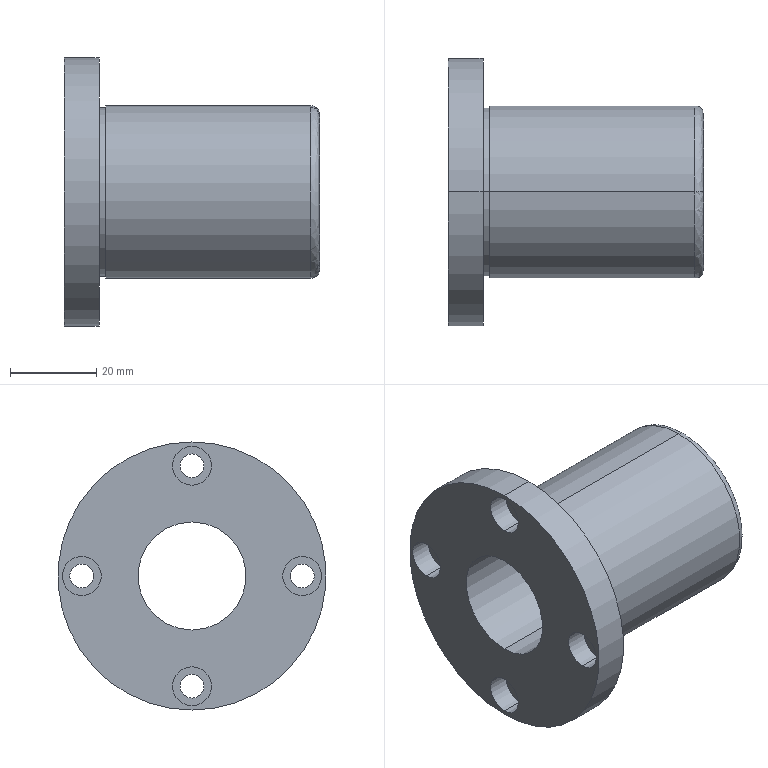Part | SolidWorks | features BaseBody 1 | 1 solid | 34 faces | box 59 x 62 x 62 mm | volume 57509 mm3 | cylinder 24 | plane 8 | spline 2 | commonest cylinder face diameters 5.5 x8 9 x8 25 x2 39 x2 40 x2 62 x2
STEP:
#1=CARTESIAN_POINT('',(57.,0.,-20.));
#2=VERTEX_POINT('',#1);
#3=CARTESIAN_POINT('',(57.,0.,20.));
#4=VERTEX_POINT('',#3);
#5=CARTESIAN_POINT('',(57.,0.,0.));
#6=DIRECTION('',(-1.,0.,0.));
#7=DIRECTION('',(0.,0.,-1.));
#8=AXIS2_PLACEMENT_3D('',#5,#6,#7);
#9=CIRCLE('',#8,20.);
#10=EDGE_CURVE('',#2,#4,#9,.T.);
#11=ORIENTED_EDGE('',*,*,#10,.F.);
#12=CARTESIAN_POINT('',(59.,0.,-18.));
#13=VERTEX_POINT('',#12);
#14=CARTESIAN_POINT('',(57.,0.,-18.));
#15=DIRECTION('',(0.,-1.,0.));
#16=DIRECTION('',(0.,0.,-1.));
#17=AXIS2_PLACEMENT_3D('',#14,#15,#16);
#18=CIRCLE('',#17,2.);
#19=EDGE_CURVE('',#2,#13,#18,.T.);
#20=ORIENTED_EDGE('',*,*,#19,.T.);
#21=CARTESIAN_POINT('',(59.,0.,18.));
#22=VERTEX_POINT('',#21);
#23=CARTESIAN_POINT('',(59.,0.,-18.));
#24=CARTESIAN_POINT('',(59.,-36.,-18.));
#25=CARTESIAN_POINT('',(59.,-36.,18.));
#26=CARTESIAN_POINT('',(59.,0.,18.));
#27=(BOUNDED_CURVE()B_SPLINE_CURVE(3,(#23,#24,#25,#26),.UNSPECIFIED.,.F.,.F.)B_SPLINE_CURVE_WITH_KNOTS((4,4),(0.,1.),.UNSPECIFIED.)CURVE()GEOMETRIC_REPRESENTATION_ITEM()RATIONAL_B_SPLINE_CURVE((1.,0.3333,0.3333,1.))REPRESENTATION_ITEM(''));
#28=EDGE_CURVE('',#13,#22,#27,.T.);
#29=ORIENTED_EDGE('',*,*,#28,.T.);
#30=CARTESIAN_POINT('',(57.,0.,18.));
#31=DIRECTION('',(0.,1.,0.));
#32=DIRECTION('',(0.,0.,1.));
#33=AXIS2_PLACEMENT_3D('',#30,#31,#32);
#34=CIRCLE('',#33,2.);
#35=EDGE_CURVE('',#4,#22,#34,.T.);
#36=ORIENTED_EDGE('',*,*,#35,.F.);
#37=EDGE_LOOP('',(#11,#20,#29,#36));
#38=FACE_OUTER_BOUND('',#37,.T.);
#39=CARTESIAN_POINT('',(57.,0.,-20.));
#40=CARTESIAN_POINT('',(57.,-40.,-20.));
#41=CARTESIAN_POINT('',(57.,-40.,20.));
#42=CARTESIAN_POINT('',(57.,0.,20.));
#43=CARTESIAN_POINT('',(58.172,0.,-20.));
#44=CARTESIAN_POINT('',(58.172,-40.,-20.));
#45=CARTESIAN_POINT('',(58.172,-40.,20.));
#46=CARTESIAN_POINT('',(58.172,0.,20.));
#47=CARTESIAN_POINT('',(59.,0.,-19.172));
#48=CARTESIAN_POINT('',(59.,-38.343,-19.172));
#49=CARTESIAN_POINT('',(59.,-38.343,19.172));
#50=CARTESIAN_POINT('',(59.,0.,19.172));
#51=CARTESIAN_POINT('',(59.,0.,-18.));
#52=CARTESIAN_POINT('',(59.,-36.,-18.));
#53=CARTESIAN_POINT('',(59.,-36.,18.));
#54=CARTESIAN_POINT('',(59.,0.,18.));
#55=(BOUNDED_SURFACE()B_SPLINE_SURFACE(3,3,((#39,#40,#41,#42),(#43,#44,#45,#46),(#47,#48,#49,#50),(#51,#52,#53,#54)),.UNSPECIFIED.,.F.,.F.,.T.)B_SPLINE_SURFACE_WITH_KNOTS((4,4),(4,4),(0.,1.),(0.,1.),.UNSPECIFIED.)GEOMETRIC_REPRESENTATION_ITEM()RATIONAL_B_SPLINE_SURFACE(((1.,0.3333,0.3333,1.),(0.8047,0.2682,0.2682,0.8047),(0.8047,0.2682,0.2682,0.8047),(1.,0.3333,0.3333,1.)))REPRESENTATION_ITEM('')SURFACE());
#56=ADVANCED_FACE('',(#38),#55,.T.);
#57=CARTESIAN_POINT('',(9.5,0.,-20.));
#58=VERTEX_POINT('',#57);
#59=CARTESIAN_POINT('',(9.5,0.,20.));
#60=VERTEX_POINT('',#59);
#61=CARTESIAN_POINT('',(9.5,0.,0.));
#62=DIRECTION('',(1.,0.,0.));
#63=DIRECTION('',(0.,0.,-1.));
#64=AXIS2_PLACEMENT_3D('',#61,#62,#63);
#65=CIRCLE('',#64,20.);
#66=EDGE_CURVE('',#58,#60,#65,.T.);
#67=ORIENTED_EDGE('',*,*,#66,.T.);
#68=CARTESIAN_POINT('',(33.25,0.,20.));
#69=DIRECTION('',(1.,0.,0.));
#70=VECTOR('',#69,1000.);
#71=LINE('',#68,#70);
#72=EDGE_CURVE('',#60,#4,#71,.T.);
#73=ORIENTED_EDGE('',*,*,#72,.T.);
#74=CARTESIAN_POINT('',(57.,0.,0.));
#75=DIRECTION('',(-1.,0.,0.));
#76=DIRECTION('',(0.,0.,-1.));
#77=AXIS2_PLACEMENT_3D('',#74,#75,#76);
#78=CIRCLE('',#77,20.);
#79=EDGE_CURVE('',#4,#2,#78,.T.);
#80=ORIENTED_EDGE('',*,*,#79,.T.);
#81=CARTESIAN_POINT('',(33.25,0.,-20.));
#82=DIRECTION('',(1.,0.,0.));
#83=VECTOR('',#82,1000.);
#84=LINE('',#81,#83);
#85=EDGE_CURVE('',#58,#2,#84,.T.);
#86=ORIENTED_EDGE('',*,*,#85,.F.);
#87=EDGE_LOOP('',(#67,#73,#80,#86));
#88=FACE_OUTER_BOUND('',#87,.T.);
#89=CARTESIAN_POINT('',(33.25,0.,0.));
#90=DIRECTION('',(1.,0.,0.));
#91=DIRECTION('',(0.,0.,-1.));
#92=AXIS2_PLACEMENT_3D('',#89,#90,#91);
#93=CYLINDRICAL_SURFACE('',#92,20.);
#94=ADVANCED_FACE('',(#88),#93,.T.);
#95=CARTESIAN_POINT('',(8.,0.,-19.5));
#96=VERTEX_POINT('',#95);
#97=CARTESIAN_POINT('',(8.,0.,19.5));
#98=VERTEX_POINT('',#97);
#99=CARTESIAN_POINT('',(8.,0.,0.));
#100=DIRECTION('',(1.,0.,0.));
#101=DIRECTION('',(0.,0.,-1.));
#102=AXIS2_PLACEMENT_3D('',#99,#100,#101);
#103=CIRCLE('',#102,19.5);
#104=EDGE_CURVE('',#96,#98,#103,.T.);
#105=ORIENTED_EDGE('',*,*,#104,.T.);
#106=CARTESIAN_POINT('',(9.5,0.,19.5));
#107=VERTEX_POINT('',#106);
#108=CARTESIAN_POINT('',(8.75,0.,19.5));
#109=DIRECTION('',(1.,0.,0.));
#110=VECTOR('',#109,1000.);
#111=LINE('',#108,#110);
#112=EDGE_CURVE('',#98,#107,#111,.T.);
#113=ORIENTED_EDGE('',*,*,#112,.T.);
#114=CARTESIAN_POINT('',(9.5,0.,-19.5));
#115=VERTEX_POINT('',#114);
#116=CARTESIAN_POINT('',(9.5,0.,0.));
#117=DIRECTION('',(1.,0.,0.));
#118=DIRECTION('',(0.,0.,-1.));
#119=AXIS2_PLACEMENT_3D('',#116,#117,#118);
#120=CIRCLE('',#119,19.5);
#121=EDGE_CURVE('',#115,#107,#120,.T.);
#122=ORIENTED_EDGE('',*,*,#121,.F.);
#123=CARTESIAN_POINT('',(8.75,0.,-19.5));
#124=DIRECTION('',(1.,0.,0.));
#125=VECTOR('',#124,1000.);
#126=LINE('',#123,#125);
#127=EDGE_CURVE('',#96,#115,#126,.T.);
#128=ORIENTED_EDGE('',*,*,#127,.F.);
#129=EDGE_LOOP('',(#105,#113,#122,#128));
#130=FACE_OUTER_BOUND('',#129,.T.);
#131=CARTESIAN_POINT('',(8.75,0.,0.));
#132=DIRECTION('',(1.,0.,0.));
#133=DIRECTION('',(0.,0.,-1.));
#134=AXIS2_PLACEMENT_3D('',#131,#132,#133);
#135=CYLINDRICAL_SURFACE('',#134,19.5);
#136=ADVANCED_FACE('',(#130),#135,.T.);
#137=CARTESIAN_POINT('',(0.,0.,12.5));
#138=VERTEX_POINT('',#137);
#139=CARTESIAN_POINT('',(0.,0.,-12.5));
#140=VERTEX_POINT('',#139);
#141=CARTESIAN_POINT('',(0.,0.,0.));
#142=DIRECTION('',(1.,0.,0.));
#143=DIRECTION('',(0.,0.,-1.));
#144=AXIS2_PLACEMENT_3D('',#141,#142,#143);
#145=CIRCLE('',#144,12.5);
#146=EDGE_CURVE('',#138,#140,#145,.T.);
#147=ORIENTED_EDGE('',*,*,#146,.F.);
#148=CARTESIAN_POINT('',(59.,0.,12.5));
#149=VERTEX_POINT('',#148);
#150=CARTESIAN_POINT('',(29.5,0.,12.5));
#151=DIRECTION('',(1.,0.,0.));
#152=VECTOR('',#151,1000.);
#153=LINE('',#150,#152);
#154=EDGE_CURVE('',#138,#149,#153,.T.);
#155=ORIENTED_EDGE('',*,*,#154,.T.);
#156=CARTESIAN_POINT('',(59.,0.,-12.5));
#157=VERTEX_POINT('',#156);
#158=CARTESIAN_POINT('',(59.,0.,0.));
#159=DIRECTION('',(-1.,0.,0.));
#160=DIRECTION('',(0.,0.,-1.));
#161=AXIS2_PLACEMENT_3D('',#158,#159,#160);
#162=CIRCLE('',#161,12.5);
#163=EDGE_CURVE('',#157,#149,#162,.T.);
#164=ORIENTED_EDGE('',*,*,#163,.F.);
#165=CARTESIAN_POINT('',(29.5,0.,-12.5));
#166=DIRECTION('',(1.,0.,0.));
#167=VECTOR('',#166,1000.);
#168=LINE('',#165,#167);
#169=EDGE_CURVE('',#140,#157,#168,.T.);
#170=ORIENTED_EDGE('',*,*,#169,.F.);
#171=EDGE_LOOP('',(#147,#155,#164,#170));
#172=FACE_OUTER_BOUND('',#171,.T.);
#173=CARTESIAN_POINT('',(29.5,0.,0.));
#174=DIRECTION('',(1.,0.,0.));
#175=DIRECTION('',(0.,0.,-1.));
#176=AXIS2_PLACEMENT_3D('',#173,#174,#175);
#177=CYLINDRICAL_SURFACE('',#176,12.5);
#178=ADVANCED_FACE('',(#172),#177,.F.);
#179=CARTESIAN_POINT('',(0.,0.,31.));
#180=VERTEX_POINT('',#179);
#181=CARTESIAN_POINT('',(0.,0.,-31.));
#182=VERTEX_POINT('',#181);
#183=CARTESIAN_POINT('',(0.,0.,0.));
#184=DIRECTION('',(-1.,0.,0.));
#185=DIRECTION('',(0.,0.,-1.));
#186=AXIS2_PLACEMENT_3D('',#183,#184,#185);
#187=CIRCLE('',#186,31.);
#188=EDGE_CURVE('',#180,#182,#187,.T.);
#189=ORIENTED_EDGE('',*,*,#188,.F.);
#190=CARTESIAN_POINT('',(8.,0.,31.));
#191=VERTEX_POINT('',#190);
#192=CARTESIAN_POINT('',(4.,0.,31.));
#193=DIRECTION('',(1.,0.,0.));
#194=VECTOR('',#193,1000.);
#195=LINE('',#192,#194);
#196=EDGE_CURVE('',#180,#191,#195,.T.);
#197=ORIENTED_EDGE('',*,*,#196,.T.);
#198=CARTESIAN_POINT('',(8.,0.,-31.));
#199=VERTEX_POINT('',#198);
#200=CARTESIAN_POINT('',(8.,0.,0.));
#201=DIRECTION('',(1.,0.,0.));
#202=DIRECTION('',(0.,0.,-1.));
#203=AXIS2_PLACEMENT_3D('',#200,#201,#202);
#204=CIRCLE('',#203,31.);
#205=EDGE_CURVE('',#199,#191,#204,.T.);
#206=ORIENTED_EDGE('',*,*,#205,.F.);
#207=CARTESIAN_POINT('',(4.,0.,-31.));
#208=DIRECTION('',(1.,0.,0.));
#209=VECTOR('',#208,1000.);
#210=LINE('',#207,#209);
#211=EDGE_CURVE('',#182,#199,#210,.T.);
#212=ORIENTED_EDGE('',*,*,#211,.F.);
#213=EDGE_LOOP('',(#189,#197,#206,#212));
#214=FACE_OUTER_BOUND('',#213,.T.);
#215=CARTESIAN_POINT('',(4.,0.,0.));
#216=DIRECTION('',(1.,0.,0.));
#217=DIRECTION('',(0.,0.,-1.));
#218=AXIS2_PLACEMENT_3D('',#215,#216,#217);
#219=CYLINDRICAL_SURFACE('',#218,31.);
#220=ADVANCED_FACE('',(#214),#219,.T.);
#221=CARTESIAN_POINT('',(5.1,25.5,2.75));
#222=VERTEX_POINT('',#221);
#223=CARTESIAN_POINT('',(5.1,25.5,-2.75));
#224=VERTEX_POINT('',#223);
#225=CARTESIAN_POINT('',(5.1,25.5,0.));
#226=DIRECTION('',(1.,0.,0.));
#227=DIRECTION('',(0.,0.,-1.));
#228=AXIS2_PLACEMENT_3D('',#225,#226,#227);
#229=CIRCLE('',#228,2.75);
#230=EDGE_CURVE('',#222,#224,#229,.T.);
#231=ORIENTED_EDGE('',*,*,#230,.F.);
#232=CARTESIAN_POINT('',(8.,25.5,2.75));
#233=VERTEX_POINT('',#232);
#234=CARTESIAN_POINT('',(6.55,25.5,2.75));
#235=DIRECTION('',(1.,0.,0.));
#236=VECTOR('',#235,1000.);
#237=LINE('',#234,#236);
#238=EDGE_CURVE('',#222,#233,#237,.T.);
#239=ORIENTED_EDGE('',*,*,#238,.T.);
#240=CARTESIAN_POINT('',(8.,25.5,-2.75));
#241=VERTEX_POINT('',#240);
#242=CARTESIAN_POINT('',(8.,25.5,0.));
#243=DIRECTION('',(-1.,0.,0.));
#244=DIRECTION('',(0.,0.,-1.));
#245=AXIS2_PLACEMENT_3D('',#242,#243,#244);
#246=CIRCLE('',#245,2.75);
#247=EDGE_CURVE('',#241,#233,#246,.T.);
#248=ORIENTED_EDGE('',*,*,#247,.F.);
#249=CARTESIAN_POINT('',(6.55,25.5,-2.75));
#250=DIRECTION('',(1.,0.,0.));
#251=VECTOR('',#250,1000.);
#252=LINE('',#249,#251);
#253=EDGE_CURVE('',#224,#241,#252,.T.);
#254=ORIENTED_EDGE('',*,*,#253,.F.);
#255=EDGE_LOOP('',(#231,#239,#248,#254));
#256=FACE_OUTER_BOUND('',#255,.T.);
#257=CARTESIAN_POINT('',(6.55,25.5,0.));
#258=DIRECTION('',(1.,0.,0.));
#259=DIRECTION('',(0.,0.,-1.));
#260=AXIS2_PLACEMENT_3D('',#257,#258,#259);
#261=CYLINDRICAL_SURFACE('',#260,2.75);
#262=ADVANCED_FACE('',(#256),#261,.F.);
#263=CARTESIAN_POINT('',(5.1,-25.5,2.75));
#264=VERTEX_POINT('',#263);
#265=CARTESIAN_POINT('',(5.1,-25.5,-2.75));
#266=VERTEX_POINT('',#265);
#267=CARTESIAN_POINT('',(5.1,-25.5,0.));
#268=DIRECTION('',(1.,0.,0.));
#269=DIRECTION('',(0.,0.,-1.));
#270=AXIS2_PLACEMENT_3D('',#267,#268,#269);
#271=CIRCLE('',#270,2.75);
#272=EDGE_CURVE('',#264,#266,#271,.T.);
#273=ORIENTED_EDGE('',*,*,#272,.F.);
#274=CARTESIAN_POINT('',(8.,-25.5,2.75));
#275=VERTEX_POINT('',#274);
#276=CARTESIAN_POINT('',(6.55,-25.5,2.75));
#277=DIRECTION('',(1.,0.,0.));
#278=VECTOR('',#277,1000.);
#279=LINE('',#276,#278);
#280=EDGE_CURVE('',#264,#275,#279,.T.);
#281=ORIENTED_EDGE('',*,*,#280,.T.);
#282=CARTESIAN_POINT('',(8.,-25.5,-2.75));
#283=VERTEX_POINT('',#282);
#284=CARTESIAN_POINT('',(8.,-25.5,0.));
#285=DIRECTION('',(-1.,0.,0.));
#286=DIRECTION('',(0.,0.,-1.));
#287=AXIS2_PLACEMENT_3D('',#284,#285,#286);
#288=CIRCLE('',#287,2.75);
#289=EDGE_CURVE('',#283,#275,#288,.T.);
#290=ORIENTED_EDGE('',*,*,#289,.F.);
#291=CARTESIAN_POINT('',(6.55,-25.5,-2.75));
#292=DIRECTION('',(1.,0.,0.));
#293=VECTOR('',#292,1000.);
#294=LINE('',#291,#293);
#295=EDGE_CURVE('',#266,#283,#294,.T.);
#296=ORIENTED_EDGE('',*,*,#295,.F.);
#297=EDGE_LOOP('',(#273,#281,#290,#296));
#298=FACE_OUTER_BOUND('',#297,.T.);
#299=CARTESIAN_POINT('',(6.55,-25.5,0.));
#300=DIRECTION('',(1.,0.,0.));
#301=DIRECTION('',(0.,0.,-1.));
#302=AXIS2_PLACEMENT_3D('',#299,#300,#301);
#303=CYLINDRICAL_SURFACE('',#302,2.75);
#304=ADVANCED_FACE('',(#298),#303,.F.);
#305=CARTESIAN_POINT('',(5.1,0.,-22.75));
#306=VERTEX_POINT('',#305);
#307=CARTESIAN_POINT('',(5.1,0.,-28.25));
#308=VERTEX_POINT('',#307);
#309=CARTESIAN_POINT('',(5.1,0.,-25.5));
#310=DIRECTION('',(1.,0.,0.));
#311=DIRECTION('',(0.,0.,-1.));
#312=AXIS2_PLACEMENT_3D('',#309,#310,#311);
#313=CIRCLE('',#312,2.75);
#314=EDGE_CURVE('',#306,#308,#313,.T.);
#315=ORIENTED_EDGE('',*,*,#314,.F.);
#316=CARTESIAN_POINT('',(8.,0.,-22.75));
#317=VERTEX_POINT('',#316);
#318=CARTESIAN_POINT('',(6.55,0.,-22.75));
#319=DIRECTION('',(1.,0.,0.));
#320=VECTOR('',#319,1000.);
#321=LINE('',#318,#320);
#322=EDGE_CURVE('',#306,#317,#321,.T.);
#323=ORIENTED_EDGE('',*,*,#322,.T.);
#324=CARTESIAN_POINT('',(8.,0.,-28.25));
#325=VERTEX_POINT('',#324);
#326=CARTESIAN_POINT('',(8.,0.,-25.5));
#327=DIRECTION('',(-1.,0.,0.));
#328=DIRECTION('',(0.,0.,-1.));
#329=AXIS2_PLACEMENT_3D('',#326,#327,#328);
#330=CIRCLE('',#329,2.75);
#331=EDGE_CURVE('',#325,#317,#330,.T.);
#332=ORIENTED_EDGE('',*,*,#331,.F.);
#333=CARTESIAN_POINT('',(6.55,0.,-28.25));
#334=DIRECTION('',(1.,0.,0.));
#335=VECTOR('',#334,1000.);
#336=LINE('',#333,#335);
#337=EDGE_CURVE('',#308,#325,#336,.T.);
#338=ORIENTED_EDGE('',*,*,#337,.F.);
#339=EDGE_LOOP('',(#315,#323,#332,#338));
#340=FACE_OUTER_BOUND('',#339,.T.);
#341=CARTESIAN_POINT('',(6.55,0.,-25.5));
#342=DIRECTION('',(1.,0.,0.));
#343=DIRECTION('',(0.,0.,-1.));
#344=AXIS2_PLACEMENT_3D('',#341,#342,#343);
#345=CYLINDRICAL_SURFACE('',#344,2.75);
#346=ADVANCED_FACE('',(#340),#345,.F.);
#347=CARTESIAN_POINT('',(5.1,0.,28.25));
#348=VERTEX_POINT('',#347);
#349=CARTESIAN_POINT('',(5.1,0.,22.75));
#350=VERTEX_POINT('',#349);
#351=CARTESIAN_POINT('',(5.1,0.,25.5));
#352=DIRECTION('',(1.,0.,0.));
#353=DIRECTION('',(0.,0.,-1.));
#354=AXIS2_PLACEMENT_3D('',#351,#352,#353);
#355=CIRCLE('',#354,2.75);
#356=EDGE_CURVE('',#348,#350,#355,.T.);
#357=ORIENTED_EDGE('',*,*,#356,.F.);
#358=CARTESIAN_POINT('',(8.,0.,28.25));
#359=VERTEX_POINT('',#358);
#360=CARTESIAN_POINT('',(6.55,0.,28.25));
#361=DIRECTION('',(1.,0.,0.));
#362=VECTOR('',#361,1000.);
#363=LINE('',#360,#362);
#364=EDGE_CURVE('',#348,#359,#363,.T.);
#365=ORIENTED_EDGE('',*,*,#364,.T.);
#366=CARTESIAN_POINT('',(8.,0.,22.75));
#367=VERTEX_POINT('',#366);
#368=CARTESIAN_POINT('',(8.,0.,25.5));
#369=DIRECTION('',(-1.,0.,0.));
#370=DIRECTION('',(0.,0.,-1.));
#371=AXIS2_PLACEMENT_3D('',#368,#369,#370);
#372=CIRCLE('',#371,2.75);
#373=EDGE_CURVE('',#367,#359,#372,.T.);
#374=ORIENTED_EDGE('',*,*,#373,.F.);
#375=CARTESIAN_POINT('',(6.55,0.,22.75));
#376=DIRECTION('',(1.,0.,0.));
#377=VECTOR('',#376,1000.);
#378=LINE('',#375,#377);
#379=EDGE_CURVE('',#350,#367,#378,.T.);
#380=ORIENTED_EDGE('',*,*,#379,.F.);
#381=EDGE_LOOP('',(#357,#365,#374,#380));
#382=FACE_OUTER_BOUND('',#381,.T.);
#383=CARTESIAN_POINT('',(6.55,0.,25.5));
#384=DIRECTION('',(1.,0.,0.));
#385=DIRECTION('',(0.,0.,-1.));
#386=AXIS2_PLACEMENT_3D('',#383,#384,#385);
#387=CYLINDRICAL_SURFACE('',#386,2.75);
#388=ADVANCED_FACE('',(#382),#387,.F.);
#389=CARTESIAN_POINT('',(0.,25.5,4.5));
#390=VERTEX_POINT('',#389);
#391=CARTESIAN_POINT('',(0.,25.5,-4.5));
#392=VERTEX_POINT('',#391);
#393=CARTESIAN_POINT('',(0.,25.5,0.));
#394=DIRECTION('',(1.,0.,0.));
#395=DIRECTION('',(0.,0.,-1.));
#396=AXIS2_PLACEMENT_3D('',#393,#394,#395);
#397=CIRCLE('',#396,4.5);
#398=EDGE_CURVE('',#390,#392,#397,.T.);
#399=ORIENTED_EDGE('',*,*,#398,.F.);
#400=CARTESIAN_POINT('',(5.1,25.5,4.5));
#401=VERTEX_POINT('',#400);
#402=CARTESIAN_POINT('',(2.55,25.5,4.5));
#403=DIRECTION('',(1.,0.,0.));
#404=VECTOR('',#403,1000.);
#405=LINE('',#402,#404);
#406=EDGE_CURVE('',#390,#401,#405,.T.);
#407=ORIENTED_EDGE('',*,*,#406,.T.);
#408=CARTESIAN_POINT('',(5.1,25.5,-4.5));
#409=VERTEX_POINT('',#408);
#410=CARTESIAN_POINT('',(5.1,25.5,0.));
#411=DIRECTION('',(-1.,0.,0.));
#412=DIRECTION('',(0.,0.,-1.));
#413=AXIS2_PLACEMENT_3D('',#410,#411,#412);
#414=CIRCLE('',#413,4.5);
#415=EDGE_CURVE('',#409,#401,#414,.T.);
#416=ORIENTED_EDGE('',*,*,#415,.F.);
#417=CARTESIAN_POINT('',(2.55,25.5,-4.5));
#418=DIRECTION('',(1.,0.,0.));
#419=VECTOR('',#418,1000.);
#420=LINE('',#417,#419);
#421=EDGE_CURVE('',#392,#409,#420,.T.);
#422=ORIENTED_EDGE('',*,*,#421,.F.);
#423=EDGE_LOOP('',(#399,#407,#416,#422));
#424=FACE_OUTER_BOUND('',#423,.T.);
#425=CARTESIAN_POINT('',(2.55,25.5,0.));
#426=DIRECTION('',(1.,0.,0.));
#427=DIRECTION('',(0.,0.,-1.));
#428=AXIS2_PLACEMENT_3D('',#425,#426,#427);
#429=CYLINDRICAL_SURFACE('',#428,4.5);
#430=ADVANCED_FACE('',(#424),#429,.F.);
#431=CARTESIAN_POINT('',(0.,-25.5,4.5));
#432=VERTEX_POINT('',#431);
#433=CARTESIAN_POINT('',(0.,-25.5,-4.5));
#434=VERTEX_POINT('',#433);
#435=CARTESIAN_POINT('',(0.,-25.5,0.));
#436=DIRECTION('',(1.,0.,0.));
#437=DIRECTION('',(0.,0.,-1.));
#438=AXIS2_PLACEMENT_3D('',#435,#436,#437);
#439=CIRCLE('',#438,4.5);
#440=EDGE_CURVE('',#432,#434,#439,.T.);
#441=ORIENTED_EDGE('',*,*,#440,.F.);
#442=CARTESIAN_POINT('',(5.1,-25.5,4.5));
#443=VERTEX_POINT('',#442);
#444=CARTESIAN_POINT('',(2.55,-25.5,4.5));
#445=DIRECTION('',(1.,0.,0.));
#446=VECTOR('',#445,1000.);
#447=LINE('',#444,#446);
#448=EDGE_CURVE('',#432,#443,#447,.T.);
#449=ORIENTED_EDGE('',*,*,#448,.T.);
#450=CARTESIAN_POINT('',(5.1,-25.5,-4.5));
#451=VERTEX_POINT('',#450);
#452=CARTESIAN_POINT('',(5.1,-25.5,0.));
#453=DIRECTION('',(-1.,0.,0.));
#454=DIRECTION('',(0.,0.,-1.));
#455=AXIS2_PLACEMENT_3D('',#452,#453,#454);
#456=CIRCLE('',#455,4.5);
#457=EDGE_CURVE('',#451,#443,#456,.T.);
#458=ORIENTED_EDGE('',*,*,#457,.F.);
#459=CARTESIAN_POINT('',(2.55,-25.5,-4.5));
#460=DIRECTION('',(1.,0.,0.));
#461=VECTOR('',#460,1000.);
#462=LINE('',#459,#461);
#463=EDGE_CURVE('',#434,#451,#462,.T.);
#464=ORIENTED_EDGE('',*,*,#463,.F.);
#465=EDGE_LOOP('',(#441,#449,#458,#464));
#466=FACE_OUTER_BOUND('',#465,.T.);
#467=CARTESIAN_POINT('',(2.55,-25.5,0.));
#468=DIRECTION('',(1.,0.,0.));
#469=DIRECTION('',(0.,0.,-1.));
#470=AXIS2_PLACEMENT_3D('',#467,#468,#469);
#471=CYLINDRICAL_SURFACE('',#470,4.5);
#472=ADVANCED_FACE('',(#466),#471,.F.);
#473=CARTESIAN_POINT('',(0.,0.,-21.));
#474=VERTEX_POINT('',#473);
#475=CARTESIAN_POINT('',(0.,0.,-30.));
#476=VERTEX_POINT('',#475);
#477=CARTESIAN_POINT('',(0.,0.,-25.5));
#478=DIRECTION('',(1.,0.,0.));
#479=DIRECTION('',(0.,0.,-1.));
#480=AXIS2_PLACEMENT_3D('',#477,#478,#479);
#481=CIRCLE('',#480,4.5);
#482=EDGE_CURVE('',#474,#476,#481,.T.);
#483=ORIENTED_EDGE('',*,*,#482,.F.);
#484=CARTESIAN_POINT('',(5.1,0.,-21.));
#485=VERTEX_POINT('',#484);
#486=CARTESIAN_POINT('',(2.55,0.,-21.));
#487=DIRECTION('',(1.,0.,0.));
#488=VECTOR('',#487,1000.);
#489=LINE('',#486,#488);
#490=EDGE_CURVE('',#474,#485,#489,.T.);
#491=ORIENTED_EDGE('',*,*,#490,.T.);
#492=CARTESIAN_POINT('',(5.1,0.,-30.));
#493=VERTEX_POINT('',#492);
#494=CARTESIAN_POINT('',(5.1,0.,-25.5));
#495=DIRECTION('',(-1.,0.,0.));
#496=DIRECTION('',(0.,0.,-1.));
#497=AXIS2_PLACEMENT_3D('',#494,#495,#496);
#498=CIRCLE('',#497,4.5);
#499=EDGE_CURVE('',#493,#485,#498,.T.);
#500=ORIENTED_EDGE('',*,*,#499,.F.);
#501=CARTESIAN_POINT('',(2.55,0.,-30.));
#502=DIRECTION('',(1.,0.,0.));
#503=VECTOR('',#502,1000.);
#504=LINE('',#501,#503);
#505=EDGE_CURVE('',#476,#493,#504,.T.);
#506=ORIENTED_EDGE('',*,*,#505,.F.);
#507=EDGE_LOOP('',(#483,#491,#500,#506));
#508=FACE_OUTER_BOUND('',#507,.T.);
#509=CARTESIAN_POINT('',(2.55,0.,-25.5));
#510=DIRECTION('',(1.,0.,0.));
#511=DIRECTION('',(0.,0.,-1.));
#512=AXIS2_PLACEMENT_3D('',#509,#510,#511);
#513=CYLINDRICAL_SURFACE('',#512,4.5);
#514=ADVANCED_FACE('',(#508),#513,.F.);
#515=CARTESIAN_POINT('',(0.,0.,30.));
#516=VERTEX_POINT('',#515);
#517=CARTESIAN_POINT('',(0.,0.,21.));
#518=VERTEX_POINT('',#517);
#519=CARTESIAN_POINT('',(0.,0.,25.5));
#520=DIRECTION('',(1.,0.,0.));
#521=DIRECTION('',(0.,0.,-1.));
#522=AXIS2_PLACEMENT_3D('',#519,#520,#521);
#523=CIRCLE('',#522,4.5);
#524=EDGE_CURVE('',#516,#518,#523,.T.);
#525=ORIENTED_EDGE('',*,*,#524,.F.);
#526=CARTESIAN_POINT('',(5.1,0.,30.));
#527=VERTEX_POINT('',#526);
#528=CARTESIAN_POINT('',(2.55,0.,30.));
#529=DIRECTION('',(1.,0.,0.));
#530=VECTOR('',#529,1000.);
#531=LINE('',#528,#530);
#532=EDGE_CURVE('',#516,#527,#531,.T.);
#533=ORIENTED_EDGE('',*,*,#532,.T.);
#534=CARTESIAN_POINT('',(5.1,0.,21.));
#535=VERTEX_POINT('',#534);
#536=CARTESIAN_POINT('',(5.1,0.,25.5));
#537=DIRECTION('',(-1.,0.,0.));
#538=DIRECTION('',(0.,0.,-1.));
#539=AXIS2_PLACEMENT_3D('',#536,#537,#538);
#540=CIRCLE('',#539,4.5);
#541=EDGE_CURVE('',#535,#527,#540,.T.);
#542=ORIENTED_EDGE('',*,*,#541,.F.);
#543=CARTESIAN_POINT('',(2.55,0.,21.));
#544=DIRECTION('',(1.,0.,0.));
#545=VECTOR('',#544,1000.);
#546=LINE('',#543,#545);
#547=EDGE_CURVE('',#518,#535,#546,.T.);
#548=ORIENTED_EDGE('',*,*,#547,.F.);
#549=EDGE_LOOP('',(#525,#533,#542,#548));
#550=FACE_OUTER_BOUND('',#549,.T.);
#551=CARTESIAN_POINT('',(2.55,0.,25.5));
#552=DIRECTION('',(1.,0.,0.));
#553=DIRECTION('',(0.,0.,-1.));
#554=AXIS2_PLACEMENT_3D('',#551,#552,#553);
#555=CYLINDRICAL_SURFACE('',#554,4.5);
#556=ADVANCED_FACE('',(#550),#555,.F.);
#557=ORIENTED_EDGE('',*,*,#72,.F.);
#558=CARTESIAN_POINT('',(9.5,0.,0.));
#559=DIRECTION('',(1.,0.,0.));
#560=DIRECTION('',(0.,0.,-1.));
#561=AXIS2_PLACEMENT_3D('',#558,#559,#560);
#562=CIRCLE('',#561,20.);
#563=EDGE_CURVE('',#60,#58,#562,.T.);
#564=ORIENTED_EDGE('',*,*,#563,.T.);
#565=ORIENTED_EDGE('',*,*,#85,.T.);
#566=ORIENTED_EDGE('',*,*,#10,.T.);
#567=EDGE_LOOP('',(#557,#564,#565,#566));
#568=FACE_OUTER_BOUND('',#567,.T.);
#569=CARTESIAN_POINT('',(33.25,0.,0.));
#570=DIRECTION('',(1.,0.,0.));
#571=DIRECTION('',(0.,0.,-1.));
#572=AXIS2_PLACEMENT_3D('',#569,#570,#571);
#573=CYLINDRICAL_SURFACE('',#572,20.);
#574=ADVANCED_FACE('',(#568),#573,.T.);
#575=ORIENTED_EDGE('',*,*,#19,.F.);
#576=ORIENTED_EDGE('',*,*,#79,.F.);
#577=ORIENTED_EDGE('',*,*,#35,.T.);
#578=CARTESIAN_POINT('',(59.,18.,0.));
#579=VERTEX_POINT('',#578);
#580=CARTESIAN_POINT('',(59.,0.,18.));
#581=CARTESIAN_POINT('',(59.,10.544,18.));
#582=CARTESIAN_POINT('',(59.,18.,10.544));
#583=CARTESIAN_POINT('',(59.,18.,0.));
#584=(BOUNDED_CURVE()B_SPLINE_CURVE(3,(#580,#581,#582,#583),.UNSPECIFIED.,.F.,.F.)B_SPLINE_CURVE_WITH_KNOTS((4,4),(0.,1.),.UNSPECIFIED.)CURVE()GEOMETRIC_REPRESENTATION_ITEM()RATIONAL_B_SPLINE_CURVE((1.,0.8047,0.8047,1.))REPRESENTATION_ITEM(''));
#585=EDGE_CURVE('',#22,#579,#584,.T.);
#586=ORIENTED_EDGE('',*,*,#585,.T.);
#587=CARTESIAN_POINT('',(59.,18.,0.));
#588=CARTESIAN_POINT('',(59.,18.,-10.544));
#589=CARTESIAN_POINT('',(59.,10.544,-18.));
#590=CARTESIAN_POINT('',(59.,0.,-18.));
#591=(BOUNDED_CURVE()B_SPLINE_CURVE(3,(#587,#588,#589,#590),.UNSPECIFIED.,.F.,.F.)B_SPLINE_CURVE_WITH_KNOTS((4,4),(0.,1.),.UNSPECIFIED.)CURVE()GEOMETRIC_REPRESENTATION_ITEM()RATIONAL_B_SPLINE_CURVE((1.,0.8047,0.8047,1.))REPRESENTATION_ITEM(''));
#592=EDGE_CURVE('',#579,#13,#591,.T.);
#593=ORIENTED_EDGE('',*,*,#592,.T.);
#594=EDGE_LOOP('',(#575,#576,#577,#586,#593));
#595=FACE_OUTER_BOUND('',#594,.T.);
#596=CARTESIAN_POINT('',(57.,0.,20.));
#597=CARTESIAN_POINT('',(57.,40.,20.));
#598=CARTESIAN_POINT('',(57.,40.,-20.));
#599=CARTESIAN_POINT('',(57.,0.,-20.));
#600=CARTESIAN_POINT('',(58.172,0.,20.));
#601=CARTESIAN_POINT('',(58.172,40.,20.));
#602=CARTESIAN_POINT('',(58.172,40.,-20.));
#603=CARTESIAN_POINT('',(58.172,0.,-20.));
#604=CARTESIAN_POINT('',(59.,0.,19.172));
#605=CARTESIAN_POINT('',(59.,38.343,19.172));
#606=CARTESIAN_POINT('',(59.,38.343,-19.172));
#607=CARTESIAN_POINT('',(59.,0.,-19.172));
#608=CARTESIAN_POINT('',(59.,0.,18.));
#609=CARTESIAN_POINT('',(59.,36.,18.));
#610=CARTESIAN_POINT('',(59.,36.,-18.));
#611=CARTESIAN_POINT('',(59.,0.,-18.));
#612=(BOUNDED_SURFACE()B_SPLINE_SURFACE(3,3,((#596,#597,#598,#599),(#600,#601,#602,#603),(#604,#605,#606,#607),(#608,#609,#610,#611)),.UNSPECIFIED.,.F.,.F.,.T.)B_SPLINE_SURFACE_WITH_KNOTS((4,4),(4,4),(0.,1.),(0.,1.),.UNSPECIFIED.)GEOMETRIC_REPRESENTATION_ITEM()RATIONAL_B_SPLINE_SURFACE(((1.,0.3333,0.3333,1.),(0.8047,0.2682,0.2682,0.8047),(0.8047,0.2682,0.2682,0.8047),(1.,0.3333,0.3333,1.)))REPRESENTATION_ITEM('')SURFACE());
#613=ADVANCED_FACE('',(#595),#612,.T.);
#614=ORIENTED_EDGE('',*,*,#66,.F.);
#615=ORIENTED_EDGE('',*,*,#563,.F.);
#616=EDGE_LOOP('',(#614,#615));
#617=FACE_OUTER_BOUND('',#616,.T.);
#618=ORIENTED_EDGE('',*,*,#121,.T.);
#619=CARTESIAN_POINT('',(9.5,0.,0.));
#620=DIRECTION('',(1.,0.,0.));
#621=DIRECTION('',(0.,0.,-1.));
#622=AXIS2_PLACEMENT_3D('',#619,#620,#621);
#623=CIRCLE('',#622,19.5);
#624=EDGE_CURVE('',#107,#115,#623,.T.);
#625=ORIENTED_EDGE('',*,*,#624,.T.);
#626=EDGE_LOOP('',(#618,#625));
#627=FACE_BOUND('',#626,.T.);
#628=CARTESIAN_POINT('',(9.5,19.75,0.));
#629=DIRECTION('',(-1.,0.,0.));
#630=DIRECTION('',(0.,0.,1.));
#631=AXIS2_PLACEMENT_3D('',#628,#629,#630);
#632=PLANE('',#631);
#633=ADVANCED_FACE('',(#617,#627),#632,.T.);
#634=ORIENTED_EDGE('',*,*,#163,.T.);
#635=CARTESIAN_POINT('',(59.,0.,0.));
#636=DIRECTION('',(-1.,0.,0.));
#637=DIRECTION('',(0.,0.,-1.));
#638=AXIS2_PLACEMENT_3D('',#635,#636,#637);
#639=CIRCLE('',#638,12.5);
#640=EDGE_CURVE('',#149,#157,#639,.T.);
#641=ORIENTED_EDGE('',*,*,#640,.T.);
#642=EDGE_LOOP('',(#634,#641));
#643=FACE_BOUND('',#642,.T.);
#644=ORIENTED_EDGE('',*,*,#585,.F.);
#645=ORIENTED_EDGE('',*,*,#28,.F.);
#646=ORIENTED_EDGE('',*,*,#592,.F.);
#647=EDGE_LOOP('',(#644,#645,#646));
#648=FACE_OUTER_BOUND('',#647,.T.);
#649=CARTESIAN_POINT('',(59.,15.25,0.));
#650=DIRECTION('',(1.,0.,0.));
#651=DIRECTION('',(0.,0.,-1.));
#652=AXIS2_PLACEMENT_3D('',#649,#650,#651);
#653=PLANE('',#652);
#654=ADVANCED_FACE('',(#643,#648),#653,.T.);
#655=ORIENTED_EDGE('',*,*,#112,.F.);
#656=CARTESIAN_POINT('',(8.,0.,0.));
#657=DIRECTION('',(1.,0.,0.));
#658=DIRECTION('',(0.,0.,-1.));
#659=AXIS2_PLACEMENT_3D('',#656,#657,#658);
#660=CIRCLE('',#659,19.5);
#661=EDGE_CURVE('',#98,#96,#660,.T.);
#662=ORIENTED_EDGE('',*,*,#661,.T.);
#663=ORIENTED_EDGE('',*,*,#127,.T.);
#664=ORIENTED_EDGE('',*,*,#624,.F.);
#665=EDGE_LOOP('',(#655,#662,#663,#664));
#666=FACE_OUTER_BOUND('',#665,.T.);
#667=CARTESIAN_POINT('',(8.75,0.,0.));
#668=DIRECTION('',(1.,0.,0.));
#669=DIRECTION('',(0.,0.,-1.));
#670=AXIS2_PLACEMENT_3D('',#667,#668,#669);
#671=CYLINDRICAL_SURFACE('',#670,19.5);
#672=ADVANCED_FACE('',(#666),#671,.T.);
#673=ORIENTED_EDGE('',*,*,#154,.F.);
#674=CARTESIAN_POINT('',(0.,0.,0.));
#675=DIRECTION('',(1.,0.,0.));
#676=DIRECTION('',(0.,0.,-1.));
#677=AXIS2_PLACEMENT_3D('',#674,#675,#676);
#678=CIRCLE('',#677,12.5);
#679=EDGE_CURVE('',#140,#138,#678,.T.);
#680=ORIENTED_EDGE('',*,*,#679,.F.);
#681=ORIENTED_EDGE('',*,*,#169,.T.);
#682=ORIENTED_EDGE('',*,*,#640,.F.);
#683=EDGE_LOOP('',(#673,#680,#681,#682));
#684=FACE_OUTER_BOUND('',#683,.T.);
#685=CARTESIAN_POINT('',(29.5,0.,0.));
#686=DIRECTION('',(1.,0.,0.));
#687=DIRECTION('',(0.,0.,-1.));
#688=AXIS2_PLACEMENT_3D('',#685,#686,#687);
#689=CYLINDRICAL_SURFACE('',#688,12.5);
#690=ADVANCED_FACE('',(#684),#689,.F.);
#691=ORIENTED_EDGE('',*,*,#104,.F.);
#692=ORIENTED_EDGE('',*,*,#661,.F.);
#693=EDGE_LOOP('',(#691,#692));
#694=FACE_BOUND('',#693,.T.);
#695=ORIENTED_EDGE('',*,*,#205,.T.);
#696=CARTESIAN_POINT('',(8.,0.,0.));
#697=DIRECTION('',(1.,0.,0.));
#698=DIRECTION('',(0.,0.,-1.));
#699=AXIS2_PLACEMENT_3D('',#696,#697,#698);
#700=CIRCLE('',#699,31.);
#701=EDGE_CURVE('',#191,#199,#700,.T.);
#702=ORIENTED_EDGE('',*,*,#701,.T.);
#703=EDGE_LOOP('',(#695,#702));
#704=FACE_OUTER_BOUND('',#703,.T.);
#705=ORIENTED_EDGE('',*,*,#247,.T.);
#706=CARTESIAN_POINT('',(8.,25.5,0.));
#707=DIRECTION('',(-1.,0.,0.));
#708=DIRECTION('',(0.,0.,-1.));
#709=AXIS2_PLACEMENT_3D('',#706,#707,#708);
#710=CIRCLE('',#709,2.75);
#711=EDGE_CURVE('',#233,#241,#710,.T.);
#712=ORIENTED_EDGE('',*,*,#711,.T.);
#713=EDGE_LOOP('',(#705,#712));
#714=FACE_BOUND('',#713,.T.);
#715=ORIENTED_EDGE('',*,*,#289,.T.);
#716=CARTESIAN_POINT('',(8.,-25.5,0.));
#717=DIRECTION('',(-1.,0.,0.));
#718=DIRECTION('',(0.,0.,-1.));
#719=AXIS2_PLACEMENT_3D('',#716,#717,#718);
#720=CIRCLE('',#719,2.75);
#721=EDGE_CURVE('',#275,#283,#720,.T.);
#722=ORIENTED_EDGE('',*,*,#721,.T.);
#723=EDGE_LOOP('',(#715,#722));
#724=FACE_BOUND('',#723,.T.);
#725=ORIENTED_EDGE('',*,*,#331,.T.);
#726=CARTESIAN_POINT('',(8.,0.,-25.5));
#727=DIRECTION('',(-1.,0.,0.));
#728=DIRECTION('',(0.,0.,-1.));
#729=AXIS2_PLACEMENT_3D('',#726,#727,#728);
#730=CIRCLE('',#729,2.75);
#731=EDGE_CURVE('',#317,#325,#730,.T.);
#732=ORIENTED_EDGE('',*,*,#731,.T.);
#733=EDGE_LOOP('',(#725,#732));
#734=FACE_BOUND('',#733,.T.);
#735=ORIENTED_EDGE('',*,*,#373,.T.);
#736=CARTESIAN_POINT('',(8.,0.,25.5));
#737=DIRECTION('',(-1.,0.,0.));
#738=DIRECTION('',(0.,0.,-1.));
#739=AXIS2_PLACEMENT_3D('',#736,#737,#738);
#740=CIRCLE('',#739,2.75);
#741=EDGE_CURVE('',#359,#367,#740,.T.);
#742=ORIENTED_EDGE('',*,*,#741,.T.);
#743=EDGE_LOOP('',(#735,#742));
#744=FACE_BOUND('',#743,.T.);
#745=CARTESIAN_POINT('',(8.,25.25,0.));
#746=DIRECTION('',(1.,0.,0.));
#747=DIRECTION('',(0.,0.,-1.));
#748=AXIS2_PLACEMENT_3D('',#745,#746,#747);
#749=PLANE('',#748);
#750=ADVANCED_FACE('',(#694,#704,#714,#724,#734,#744),#749,.T.);
#751=CARTESIAN_POINT('',(0.,0.,0.));
#752=DIRECTION('',(-1.,0.,0.));
#753=DIRECTION('',(0.,0.,-1.));
#754=AXIS2_PLACEMENT_3D('',#751,#752,#753);
#755=CIRCLE('',#754,31.);
#756=EDGE_CURVE('',#182,#180,#755,.T.);
#757=ORIENTED_EDGE('',*,*,#756,.T.);
#758=ORIENTED_EDGE('',*,*,#188,.T.);
#759=EDGE_LOOP('',(#757,#758));
#760=FACE_OUTER_BOUND('',#759,.T.);
#761=ORIENTED_EDGE('',*,*,#679,.T.);
#762=ORIENTED_EDGE('',*,*,#146,.T.);
#763=EDGE_LOOP('',(#761,#762));
#764=FACE_BOUND('',#763,.T.);
#765=CARTESIAN_POINT('',(0.,25.5,0.));
#766=DIRECTION('',(1.,0.,0.));
#767=DIRECTION('',(0.,0.,-1.));
#768=AXIS2_PLACEMENT_3D('',#765,#766,#767);
#769=CIRCLE('',#768,4.5);
#770=EDGE_CURVE('',#392,#390,#769,.T.);
#771=ORIENTED_EDGE('',*,*,#770,.T.);
#772=ORIENTED_EDGE('',*,*,#398,.T.);
#773=EDGE_LOOP('',(#771,#772));
#774=FACE_BOUND('',#773,.T.);
#775=CARTESIAN_POINT('',(0.,-25.5,0.));
#776=DIRECTION('',(1.,0.,0.));
#777=DIRECTION('',(0.,0.,-1.));
#778=AXIS2_PLACEMENT_3D('',#775,#776,#777);
#779=CIRCLE('',#778,4.5);
#780=EDGE_CURVE('',#434,#432,#779,.T.);
#781=ORIENTED_EDGE('',*,*,#780,.T.);
#782=ORIENTED_EDGE('',*,*,#440,.T.);
#783=EDGE_LOOP('',(#781,#782));
#784=FACE_BOUND('',#783,.T.);
#785=CARTESIAN_POINT('',(0.,0.,-25.5));
#786=DIRECTION('',(1.,0.,0.));
#787=DIRECTION('',(0.,0.,-1.));
#788=AXIS2_PLACEMENT_3D('',#785,#786,#787);
#789=CIRCLE('',#788,4.5);
#790=EDGE_CURVE('',#476,#474,#789,.T.);
#791=ORIENTED_EDGE('',*,*,#790,.T.);
#792=ORIENTED_EDGE('',*,*,#482,.T.);
#793=EDGE_LOOP('',(#791,#792));
#794=FACE_BOUND('',#793,.T.);
#795=CARTESIAN_POINT('',(0.,0.,25.5));
#796=DIRECTION('',(1.,0.,0.));
#797=DIRECTION('',(0.,0.,-1.));
#798=AXIS2_PLACEMENT_3D('',#795,#796,#797);
#799=CIRCLE('',#798,4.5);
#800=EDGE_CURVE('',#518,#516,#799,.T.);
#801=ORIENTED_EDGE('',*,*,#800,.T.);
#802=ORIENTED_EDGE('',*,*,#524,.T.);
#803=EDGE_LOOP('',(#801,#802));
#804=FACE_BOUND('',#803,.T.);
#805=CARTESIAN_POINT('',(0.,21.75,0.));
#806=DIRECTION('',(-1.,0.,0.));
#807=DIRECTION('',(0.,0.,1.));
#808=AXIS2_PLACEMENT_3D('',#805,#806,#807);
#809=PLANE('',#808);
#810=ADVANCED_FACE('',(#760,#764,#774,#784,#794,#804),#809,.T.);
#811=ORIENTED_EDGE('',*,*,#196,.F.);
#812=ORIENTED_EDGE('',*,*,#756,.F.);
#813=ORIENTED_EDGE('',*,*,#211,.T.);
#814=ORIENTED_EDGE('',*,*,#701,.F.);
#815=EDGE_LOOP('',(#811,#812,#813,#814));
#816=FACE_OUTER_BOUND('',#815,.T.);
#817=CARTESIAN_POINT('',(4.,0.,0.));
#818=DIRECTION('',(1.,0.,0.));
#819=DIRECTION('',(0.,0.,-1.));
#820=AXIS2_PLACEMENT_3D('',#817,#818,#819);
#821=CYLINDRICAL_SURFACE('',#820,31.);
#822=ADVANCED_FACE('',(#816),#821,.T.);
#823=ORIENTED_EDGE('',*,*,#238,.F.);
#824=CARTESIAN_POINT('',(5.1,25.5,0.));
#825=DIRECTION('',(1.,0.,0.));
#826=DIRECTION('',(0.,0.,-1.));
#827=AXIS2_PLACEMENT_3D('',#824,#825,#826);
#828=CIRCLE('',#827,2.75);
#829=EDGE_CURVE('',#224,#222,#828,.T.);
#830=ORIENTED_EDGE('',*,*,#829,.F.);
#831=ORIENTED_EDGE('',*,*,#253,.T.);
#832=ORIENTED_EDGE('',*,*,#711,.F.);
#833=EDGE_LOOP('',(#823,#830,#831,#832));
#834=FACE_OUTER_BOUND('',#833,.T.);
#835=CARTESIAN_POINT('',(6.55,25.5,0.));
#836=DIRECTION('',(1.,0.,0.));
#837=DIRECTION('',(0.,0.,-1.));
#838=AXIS2_PLACEMENT_3D('',#835,#836,#837);
#839=CYLINDRICAL_SURFACE('',#838,2.75);
#840=ADVANCED_FACE('',(#834),#839,.F.);
#841=ORIENTED_EDGE('',*,*,#280,.F.);
#842=CARTESIAN_POINT('',(5.1,-25.5,0.));
#843=DIRECTION('',(1.,0.,0.));
#844=DIRECTION('',(0.,0.,-1.));
#845=AXIS2_PLACEMENT_3D('',#842,#843,#844);
#846=CIRCLE('',#845,2.75);
#847=EDGE_CURVE('',#266,#264,#846,.T.);
#848=ORIENTED_EDGE('',*,*,#847,.F.);
#849=ORIENTED_EDGE('',*,*,#295,.T.);
#850=ORIENTED_EDGE('',*,*,#721,.F.);
#851=EDGE_LOOP('',(#841,#848,#849,#850));
#852=FACE_OUTER_BOUND('',#851,.T.);
#853=CARTESIAN_POINT('',(6.55,-25.5,0.));
#854=DIRECTION('',(1.,0.,0.));
#855=DIRECTION('',(0.,0.,-1.));
#856=AXIS2_PLACEMENT_3D('',#853,#854,#855);
#857=CYLINDRICAL_SURFACE('',#856,2.75);
#858=ADVANCED_FACE('',(#852),#857,.F.);
#859=ORIENTED_EDGE('',*,*,#322,.F.);
#860=CARTESIAN_POINT('',(5.1,0.,-25.5));
#861=DIRECTION('',(1.,0.,0.));
#862=DIRECTION('',(0.,0.,-1.));
#863=AXIS2_PLACEMENT_3D('',#860,#861,#862);
#864=CIRCLE('',#863,2.75);
#865=EDGE_CURVE('',#308,#306,#864,.T.);
#866=ORIENTED_EDGE('',*,*,#865,.F.);
#867=ORIENTED_EDGE('',*,*,#337,.T.);
#868=ORIENTED_EDGE('',*,*,#731,.F.);
#869=EDGE_LOOP('',(#859,#866,#867,#868));
#870=FACE_OUTER_BOUND('',#869,.T.);
#871=CARTESIAN_POINT('',(6.55,0.,-25.5));
#872=DIRECTION('',(1.,0.,0.));
#873=DIRECTION('',(0.,0.,-1.));
#874=AXIS2_PLACEMENT_3D('',#871,#872,#873);
#875=CYLINDRICAL_SURFACE('',#874,2.75);
#876=ADVANCED_FACE('',(#870),#875,.F.);
#877=ORIENTED_EDGE('',*,*,#364,.F.);
#878=CARTESIAN_POINT('',(5.1,0.,25.5));
#879=DIRECTION('',(1.,0.,0.));
#880=DIRECTION('',(0.,0.,-1.));
#881=AXIS2_PLACEMENT_3D('',#878,#879,#880);
#882=CIRCLE('',#881,2.75);
#883=EDGE_CURVE('',#350,#348,#882,.T.);
#884=ORIENTED_EDGE('',*,*,#883,.F.);
#885=ORIENTED_EDGE('',*,*,#379,.T.);
#886=ORIENTED_EDGE('',*,*,#741,.F.);
#887=EDGE_LOOP('',(#877,#884,#885,#886));
#888=FACE_OUTER_BOUND('',#887,.T.);
#889=CARTESIAN_POINT('',(6.55,0.,25.5));
#890=DIRECTION('',(1.,0.,0.));
#891=DIRECTION('',(0.,0.,-1.));
#892=AXIS2_PLACEMENT_3D('',#889,#890,#891);
#893=CYLINDRICAL_SURFACE('',#892,2.75);
#894=ADVANCED_FACE('',(#888),#893,.F.);
#895=ORIENTED_EDGE('',*,*,#406,.F.);
#896=ORIENTED_EDGE('',*,*,#770,.F.);
#897=ORIENTED_EDGE('',*,*,#421,.T.);
#898=CARTESIAN_POINT('',(5.1,25.5,0.));
#899=DIRECTION('',(-1.,0.,0.));
#900=DIRECTION('',(0.,0.,-1.));
#901=AXIS2_PLACEMENT_3D('',#898,#899,#900);
#902=CIRCLE('',#901,4.5);
#903=EDGE_CURVE('',#401,#409,#902,.T.);
#904=ORIENTED_EDGE('',*,*,#903,.F.);
#905=EDGE_LOOP('',(#895,#896,#897,#904));
#906=FACE_OUTER_BOUND('',#905,.T.);
#907=CARTESIAN_POINT('',(2.55,25.5,0.));
#908=DIRECTION('',(1.,0.,0.));
#909=DIRECTION('',(0.,0.,-1.));
#910=AXIS2_PLACEMENT_3D('',#907,#908,#909);
#911=CYLINDRICAL_SURFACE('',#910,4.5);
#912=ADVANCED_FACE('',(#906),#911,.F.);
#913=ORIENTED_EDGE('',*,*,#448,.F.);
#914=ORIENTED_EDGE('',*,*,#780,.F.);
#915=ORIENTED_EDGE('',*,*,#463,.T.);
#916=CARTESIAN_POINT('',(5.1,-25.5,0.));
#917=DIRECTION('',(-1.,0.,0.));
#918=DIRECTION('',(0.,0.,-1.));
#919=AXIS2_PLACEMENT_3D('',#916,#917,#918);
#920=CIRCLE('',#919,4.5);
#921=EDGE_CURVE('',#443,#451,#920,.T.);
#922=ORIENTED_EDGE('',*,*,#921,.F.);
#923=EDGE_LOOP('',(#913,#914,#915,#922));
#924=FACE_OUTER_BOUND('',#923,.T.);
#925=CARTESIAN_POINT('',(2.55,-25.5,0.));
#926=DIRECTION('',(1.,0.,0.));
#927=DIRECTION('',(0.,0.,-1.));
#928=AXIS2_PLACEMENT_3D('',#925,#926,#927);
#929=CYLINDRICAL_SURFACE('',#928,4.5);
#930=ADVANCED_FACE('',(#924),#929,.F.);
#931=ORIENTED_EDGE('',*,*,#490,.F.);
#932=ORIENTED_EDGE('',*,*,#790,.F.);
#933=ORIENTED_EDGE('',*,*,#505,.T.);
#934=CARTESIAN_POINT('',(5.1,0.,-25.5));
#935=DIRECTION('',(-1.,0.,0.));
#936=DIRECTION('',(0.,0.,-1.));
#937=AXIS2_PLACEMENT_3D('',#934,#935,#936);
#938=CIRCLE('',#937,4.5);
#939=EDGE_CURVE('',#485,#493,#938,.T.);
#940=ORIENTED_EDGE('',*,*,#939,.F.);
#941=EDGE_LOOP('',(#931,#932,#933,#940));
#942=FACE_OUTER_BOUND('',#941,.T.);
#943=CARTESIAN_POINT('',(2.55,0.,-25.5));
#944=DIRECTION('',(1.,0.,0.));
#945=DIRECTION('',(0.,0.,-1.));
#946=AXIS2_PLACEMENT_3D('',#943,#944,#945);
#947=CYLINDRICAL_SURFACE('',#946,4.5);
#948=ADVANCED_FACE('',(#942),#947,.F.);
#949=ORIENTED_EDGE('',*,*,#532,.F.);
#950=ORIENTED_EDGE('',*,*,#800,.F.);
#951=ORIENTED_EDGE('',*,*,#547,.T.);
#952=CARTESIAN_POINT('',(5.1,0.,25.5));
#953=DIRECTION('',(-1.,0.,0.));
#954=DIRECTION('',(0.,0.,-1.));
#955=AXIS2_PLACEMENT_3D('',#952,#953,#954);
#956=CIRCLE('',#955,4.5);
#957=EDGE_CURVE('',#527,#535,#956,.T.);
#958=ORIENTED_EDGE('',*,*,#957,.F.);
#959=EDGE_LOOP('',(#949,#950,#951,#958));
#960=FACE_OUTER_BOUND('',#959,.T.);
#961=CARTESIAN_POINT('',(2.55,0.,25.5));
#962=DIRECTION('',(1.,0.,0.));
#963=DIRECTION('',(0.,0.,-1.));
#964=AXIS2_PLACEMENT_3D('',#961,#962,#963);
#965=CYLINDRICAL_SURFACE('',#964,4.5);
#966=ADVANCED_FACE('',(#960),#965,.F.);
#967=ORIENTED_EDGE('',*,*,#829,.T.);
#968=ORIENTED_EDGE('',*,*,#230,.T.);
#969=EDGE_LOOP('',(#967,#968));
#970=FACE_BOUND('',#969,.T.);
#971=ORIENTED_EDGE('',*,*,#415,.T.);
#972=ORIENTED_EDGE('',*,*,#903,.T.);
#973=EDGE_LOOP('',(#971,#972));
#974=FACE_OUTER_BOUND('',#973,.T.);
#975=CARTESIAN_POINT('',(5.1,29.125,0.));
#976=DIRECTION('',(1.,0.,0.));
#977=DIRECTION('',(0.,0.,-1.));
#978=AXIS2_PLACEMENT_3D('',#975,#976,#977);
#979=PLANE('',#978);
#980=ADVANCED_FACE('',(#970,#974),#979,.F.);
#981=ORIENTED_EDGE('',*,*,#847,.T.);
#982=ORIENTED_EDGE('',*,*,#272,.T.);
#983=EDGE_LOOP('',(#981,#982));
#984=FACE_BOUND('',#983,.T.);
#985=ORIENTED_EDGE('',*,*,#457,.T.);
#986=ORIENTED_EDGE('',*,*,#921,.T.);
#987=EDGE_LOOP('',(#985,#986));
#988=FACE_OUTER_BOUND('',#987,.T.);
#989=CARTESIAN_POINT('',(5.1,-21.875,0.));
#990=DIRECTION('',(1.,0.,0.));
#991=DIRECTION('',(0.,0.,-1.));
#992=AXIS2_PLACEMENT_3D('',#989,#990,#991);
#993=PLANE('',#992);
#994=ADVANCED_FACE('',(#984,#988),#993,.F.);
#995=ORIENTED_EDGE('',*,*,#865,.T.);
#996=ORIENTED_EDGE('',*,*,#314,.T.);
#997=EDGE_LOOP('',(#995,#996));
#998=FACE_BOUND('',#997,.T.);
#999=ORIENTED_EDGE('',*,*,#499,.T.);
#1000=ORIENTED_EDGE('',*,*,#939,.T.);
#1001=EDGE_LOOP('',(#999,#1000));
#1002=FACE_OUTER_BOUND('',#1001,.T.);
#1003=CARTESIAN_POINT('',(5.1,0.,-29.125));
#1004=DIRECTION('',(1.,0.,0.));
#1005=DIRECTION('',(0.,0.,-1.));
#1006=AXIS2_PLACEMENT_3D('',#1003,#1004,#1005);
#1007=PLANE('',#1006);
#1008=ADVANCED_FACE('',(#998,#1002),#1007,.F.);
#1009=ORIENTED_EDGE('',*,*,#883,.T.);
#1010=ORIENTED_EDGE('',*,*,#356,.T.);
#1011=EDGE_LOOP('',(#1009,#1010));
#1012=FACE_BOUND('',#1011,.T.);
#1013=ORIENTED_EDGE('',*,*,#541,.T.);
#1014=ORIENTED_EDGE('',*,*,#957,.T.);
#1015=EDGE_LOOP('',(#1013,#1014));
#1016=FACE_OUTER_BOUND('',#1015,.T.);
#1017=CARTESIAN_POINT('',(5.1,0.,21.875));
#1018=DIRECTION('',(1.,0.,0.));
#1019=DIRECTION('',(0.,0.,-1.));
#1020=AXIS2_PLACEMENT_3D('',#1017,#1018,#1019);
#1021=PLANE('',#1020);
#1022=ADVANCED_FACE('',(#1012,#1016),#1021,.F.);
#1023=CLOSED_SHELL('',(#56,#94,#136,#178,#220,#262,#304,#346,#388,#430,#472,#514,#556,#574,#613,#633,#654,#672,#690,#750,#810,#822,#840,#858,#876,#894,#912,#930,#948,#966,#980,#994,#1008,#1022));
#1024=MANIFOLD_SOLID_BREP('',#1023);
#1025=CARTESIAN_POINT('',(0.,0.,0.));
#1026=DIRECTION('',(0.,0.,1.));
#1027=DIRECTION('',(1.,0.,0.));
#1028=AXIS2_PLACEMENT_3D('',#1025,#1026,#1027);
#1029=(LENGTH_UNIT()NAMED_UNIT(*)SI_UNIT(.MILLI.,.METRE.));
#1030=UNCERTAINTY_MEASURE_WITH_UNIT(LENGTH_MEASURE(0.00001),#1029,'','');
#1031=(NAMED_UNIT(*)PLANE_ANGLE_UNIT()SI_UNIT($,.RADIAN.));
#1032=(NAMED_UNIT(*)SI_UNIT($,.STERADIAN.)SOLID_ANGLE_UNIT());
#1033=(GEOMETRIC_REPRESENTATION_CONTEXT(3)GLOBAL_UNCERTAINTY_ASSIGNED_CONTEXT((#1030))GLOBAL_UNIT_ASSIGNED_CONTEXT((#1029,#1031,#1032))REPRESENTATION_CONTEXT('',''));
#1034=ADVANCED_BREP_SHAPE_REPRESENTATION('',(#1024,#1028),#1033);